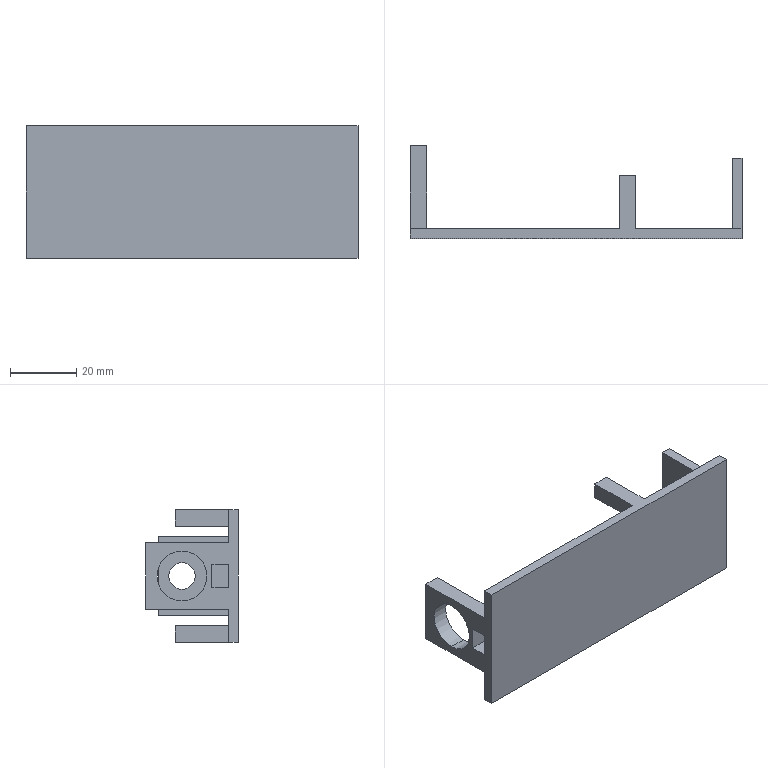Part | SolidWorks | features ICE 5, Extrusion 1 | 1 solid | 29 faces | box 100 x 28 x 40 mm | volume 15612 mm3 | plane 25 | cylinder 4 | commonest cylinder face diameters 8 x2 15 x2
STEP:
#1=CARTESIAN_POINT('',(47.,17.,4.));
#2=VERTEX_POINT('',#1);
#3=CARTESIAN_POINT('',(47.,17.,-4.));
#4=VERTEX_POINT('',#3);
#5=CARTESIAN_POINT('',(47.,17.,0.));
#6=DIRECTION('',(1.,0.,0.));
#7=DIRECTION('',(0.,0.,-1.));
#8=AXIS2_PLACEMENT_3D('',#5,#6,#7);
#9=CIRCLE('',#8,4.);
#10=EDGE_CURVE('',#2,#4,#9,.T.);
#11=ORIENTED_EDGE('',*,*,#10,.F.);
#12=CARTESIAN_POINT('',(50.,17.,4.));
#13=VERTEX_POINT('',#12);
#14=CARTESIAN_POINT('',(47.,17.,4.));
#15=DIRECTION('',(1.,0.,0.));
#16=VECTOR('',#15,1000.);
#17=LINE('',#14,#16);
#18=EDGE_CURVE('',#2,#13,#17,.T.);
#19=ORIENTED_EDGE('',*,*,#18,.T.);
#20=CARTESIAN_POINT('',(50.,17.,-4.));
#21=VERTEX_POINT('',#20);
#22=CARTESIAN_POINT('',(50.,17.,0.));
#23=DIRECTION('',(1.,0.,0.));
#24=DIRECTION('',(0.,0.,-1.));
#25=AXIS2_PLACEMENT_3D('',#22,#23,#24);
#26=CIRCLE('',#25,4.);
#27=EDGE_CURVE('',#13,#21,#26,.T.);
#28=ORIENTED_EDGE('',*,*,#27,.T.);
#29=CARTESIAN_POINT('',(47.,17.,-4.));
#30=DIRECTION('',(1.,0.,0.));
#31=VECTOR('',#30,1000.);
#32=LINE('',#29,#31);
#33=EDGE_CURVE('',#4,#21,#32,.T.);
#34=ORIENTED_EDGE('',*,*,#33,.F.);
#35=EDGE_LOOP('',(#11,#19,#28,#34));
#36=FACE_OUTER_BOUND('',#35,.T.);
#37=CARTESIAN_POINT('',(47.,17.,0.));
#38=DIRECTION('',(1.,0.,0.));
#39=DIRECTION('',(0.,0.,-1.));
#40=AXIS2_PLACEMENT_3D('',#37,#38,#39);
#41=CYLINDRICAL_SURFACE('',#40,4.);
#42=ADVANCED_FACE('',(#36),#41,.F.);
#43=CARTESIAN_POINT('',(-45.,17.,-7.5));
#44=VERTEX_POINT('',#43);
#45=CARTESIAN_POINT('',(-45.,17.,7.5));
#46=VERTEX_POINT('',#45);
#47=CARTESIAN_POINT('',(-45.,17.,0.));
#48=DIRECTION('',(-1.,0.,0.));
#49=DIRECTION('',(0.,0.,1.));
#50=AXIS2_PLACEMENT_3D('',#47,#48,#49);
#51=CIRCLE('',#50,7.5);
#52=EDGE_CURVE('',#44,#46,#51,.T.);
#53=ORIENTED_EDGE('',*,*,#52,.F.);
#54=CARTESIAN_POINT('',(-50.,17.,-7.5));
#55=VERTEX_POINT('',#54);
#56=CARTESIAN_POINT('',(-45.,17.,-7.5));
#57=DIRECTION('',(-1.,0.,0.));
#58=VECTOR('',#57,1000.);
#59=LINE('',#56,#58);
#60=EDGE_CURVE('',#44,#55,#59,.T.);
#61=ORIENTED_EDGE('',*,*,#60,.T.);
#62=CARTESIAN_POINT('',(-50.,17.,7.5));
#63=VERTEX_POINT('',#62);
#64=CARTESIAN_POINT('',(-50.,17.,0.));
#65=DIRECTION('',(-1.,0.,0.));
#66=DIRECTION('',(0.,0.,1.));
#67=AXIS2_PLACEMENT_3D('',#64,#65,#66);
#68=CIRCLE('',#67,7.5);
#69=EDGE_CURVE('',#55,#63,#68,.T.);
#70=ORIENTED_EDGE('',*,*,#69,.T.);
#71=CARTESIAN_POINT('',(-45.,17.,7.5));
#72=DIRECTION('',(-1.,0.,0.));
#73=VECTOR('',#72,1000.);
#74=LINE('',#71,#73);
#75=EDGE_CURVE('',#46,#63,#74,.T.);
#76=ORIENTED_EDGE('',*,*,#75,.F.);
#77=EDGE_LOOP('',(#53,#61,#70,#76));
#78=FACE_OUTER_BOUND('',#77,.T.);
#79=CARTESIAN_POINT('',(-45.,17.,0.));
#80=DIRECTION('',(-1.,0.,0.));
#81=DIRECTION('',(0.,0.,1.));
#82=AXIS2_PLACEMENT_3D('',#79,#80,#81);
#83=CYLINDRICAL_SURFACE('',#82,7.5);
#84=ADVANCED_FACE('',(#78),#83,.F.);
#85=CARTESIAN_POINT('',(50.,3.,20.));
#86=VERTEX_POINT('',#85);
#87=CARTESIAN_POINT('',(50.,3.,12.));
#88=VERTEX_POINT('',#87);
#89=CARTESIAN_POINT('',(50.,3.,20.));
#90=DIRECTION('',(0.,0.,-1.));
#91=VECTOR('',#90,1000.);
#92=LINE('',#89,#91);
#93=EDGE_CURVE('',#86,#88,#92,.T.);
#94=ORIENTED_EDGE('',*,*,#93,.T.);
#95=CARTESIAN_POINT('',(47.,3.,12.));
#96=VERTEX_POINT('',#95);
#97=CARTESIAN_POINT('',(0.,3.,12.));
#98=DIRECTION('',(-1.,0.,0.));
#99=VECTOR('',#98,1000.);
#100=LINE('',#97,#99);
#101=EDGE_CURVE('',#88,#96,#100,.T.);
#102=ORIENTED_EDGE('',*,*,#101,.T.);
#103=CARTESIAN_POINT('',(47.,3.,-12.));
#104=VERTEX_POINT('',#103);
#105=CARTESIAN_POINT('',(47.,3.,0.));
#106=DIRECTION('',(0.,0.,-1.));
#107=VECTOR('',#106,1000.);
#108=LINE('',#105,#107);
#109=EDGE_CURVE('',#96,#104,#108,.T.);
#110=ORIENTED_EDGE('',*,*,#109,.T.);
#111=CARTESIAN_POINT('',(50.,3.,-12.));
#112=VERTEX_POINT('',#111);
#113=CARTESIAN_POINT('',(0.,3.,-12.));
#114=DIRECTION('',(1.,0.,0.));
#115=VECTOR('',#114,1000.);
#116=LINE('',#113,#115);
#117=EDGE_CURVE('',#104,#112,#116,.T.);
#118=ORIENTED_EDGE('',*,*,#117,.T.);
#119=CARTESIAN_POINT('',(50.,3.,-20.));
#120=VERTEX_POINT('',#119);
#121=CARTESIAN_POINT('',(50.,3.,20.));
#122=DIRECTION('',(0.,0.,-1.));
#123=VECTOR('',#122,1000.);
#124=LINE('',#121,#123);
#125=EDGE_CURVE('',#112,#120,#124,.T.);
#126=ORIENTED_EDGE('',*,*,#125,.T.);
#127=CARTESIAN_POINT('',(18.,3.,-20.));
#128=VERTEX_POINT('',#127);
#129=CARTESIAN_POINT('',(-50.,3.,-20.));
#130=DIRECTION('',(-1.,0.,0.));
#131=VECTOR('',#130,1000.);
#132=LINE('',#129,#131);
#133=EDGE_CURVE('',#120,#128,#132,.T.);
#134=ORIENTED_EDGE('',*,*,#133,.T.);
#135=CARTESIAN_POINT('',(18.,3.,-15.));
#136=VERTEX_POINT('',#135);
#137=CARTESIAN_POINT('',(18.,3.,-20.));
#138=DIRECTION('',(0.,0.,-1.));
#139=VECTOR('',#138,1000.);
#140=LINE('',#137,#139);
#141=EDGE_CURVE('',#136,#128,#140,.T.);
#142=ORIENTED_EDGE('',*,*,#141,.F.);
#143=CARTESIAN_POINT('',(13.,3.,-15.));
#144=VERTEX_POINT('',#143);
#145=CARTESIAN_POINT('',(18.,3.,-15.));
#146=DIRECTION('',(-1.,0.,0.));
#147=VECTOR('',#146,1000.);
#148=LINE('',#145,#147);
#149=EDGE_CURVE('',#136,#144,#148,.T.);
#150=ORIENTED_EDGE('',*,*,#149,.T.);
#151=CARTESIAN_POINT('',(13.,3.,-20.));
#152=VERTEX_POINT('',#151);
#153=CARTESIAN_POINT('',(13.,3.,-20.));
#154=DIRECTION('',(0.,0.,-1.));
#155=VECTOR('',#154,1000.);
#156=LINE('',#153,#155);
#157=EDGE_CURVE('',#144,#152,#156,.T.);
#158=ORIENTED_EDGE('',*,*,#157,.T.);
#159=CARTESIAN_POINT('',(-50.,3.,-20.));
#160=VERTEX_POINT('',#159);
#161=CARTESIAN_POINT('',(-50.,3.,-20.));
#162=DIRECTION('',(-1.,0.,0.));
#163=VECTOR('',#162,1000.);
#164=LINE('',#161,#163);
#165=EDGE_CURVE('',#152,#160,#164,.T.);
#166=ORIENTED_EDGE('',*,*,#165,.T.);
#167=CARTESIAN_POINT('',(-50.,3.,-10.));
#168=VERTEX_POINT('',#167);
#169=CARTESIAN_POINT('',(-50.,3.,20.));
#170=DIRECTION('',(0.,0.,1.));
#171=VECTOR('',#170,1000.);
#172=LINE('',#169,#171);
#173=EDGE_CURVE('',#160,#168,#172,.T.);
#174=ORIENTED_EDGE('',*,*,#173,.T.);
#175=CARTESIAN_POINT('',(-45.,3.,-10.));
#176=VERTEX_POINT('',#175);
#177=CARTESIAN_POINT('',(-45.,3.,-10.));
#178=DIRECTION('',(-1.,0.,0.));
#179=VECTOR('',#178,1000.);
#180=LINE('',#177,#179);
#181=EDGE_CURVE('',#176,#168,#180,.T.);
#182=ORIENTED_EDGE('',*,*,#181,.F.);
#183=CARTESIAN_POINT('',(-45.,3.,-3.5));
#184=VERTEX_POINT('',#183);
#185=CARTESIAN_POINT('',(-45.,3.,-10.));
#186=DIRECTION('',(0.,0.,1.));
#187=VECTOR('',#186,1000.);
#188=LINE('',#185,#187);
#189=EDGE_CURVE('',#176,#184,#188,.T.);
#190=ORIENTED_EDGE('',*,*,#189,.T.);
#191=CARTESIAN_POINT('',(-50.,3.,-3.5));
#192=VERTEX_POINT('',#191);
#193=CARTESIAN_POINT('',(-45.,3.,-3.5));
#194=DIRECTION('',(-1.,0.,0.));
#195=VECTOR('',#194,1000.);
#196=LINE('',#193,#195);
#197=EDGE_CURVE('',#184,#192,#196,.T.);
#198=ORIENTED_EDGE('',*,*,#197,.T.);
#199=CARTESIAN_POINT('',(-50.,3.,3.5));
#200=VERTEX_POINT('',#199);
#201=CARTESIAN_POINT('',(-50.,3.,20.));
#202=DIRECTION('',(0.,0.,1.));
#203=VECTOR('',#202,1000.);
#204=LINE('',#201,#203);
#205=EDGE_CURVE('',#192,#200,#204,.T.);
#206=ORIENTED_EDGE('',*,*,#205,.T.);
#207=CARTESIAN_POINT('',(-45.,3.,3.5));
#208=VERTEX_POINT('',#207);
#209=CARTESIAN_POINT('',(-45.,3.,3.5));
#210=DIRECTION('',(-1.,0.,0.));
#211=VECTOR('',#210,1000.);
#212=LINE('',#209,#211);
#213=EDGE_CURVE('',#208,#200,#212,.T.);
#214=ORIENTED_EDGE('',*,*,#213,.F.);
#215=CARTESIAN_POINT('',(-45.,3.,10.));
#216=VERTEX_POINT('',#215);
#217=CARTESIAN_POINT('',(-45.,3.,10.));
#218=DIRECTION('',(0.,0.,1.));
#219=VECTOR('',#218,1000.);
#220=LINE('',#217,#219);
#221=EDGE_CURVE('',#208,#216,#220,.T.);
#222=ORIENTED_EDGE('',*,*,#221,.T.);
#223=CARTESIAN_POINT('',(-50.,3.,10.));
#224=VERTEX_POINT('',#223);
#225=CARTESIAN_POINT('',(-45.,3.,10.));
#226=DIRECTION('',(-1.,0.,0.));
#227=VECTOR('',#226,1000.);
#228=LINE('',#225,#227);
#229=EDGE_CURVE('',#216,#224,#228,.T.);
#230=ORIENTED_EDGE('',*,*,#229,.T.);
#231=CARTESIAN_POINT('',(-50.,3.,20.));
#232=VERTEX_POINT('',#231);
#233=CARTESIAN_POINT('',(-50.,3.,20.));
#234=DIRECTION('',(0.,0.,1.));
#235=VECTOR('',#234,1000.);
#236=LINE('',#233,#235);
#237=EDGE_CURVE('',#224,#232,#236,.T.);
#238=ORIENTED_EDGE('',*,*,#237,.T.);
#239=CARTESIAN_POINT('',(13.,3.,20.));
#240=VERTEX_POINT('',#239);
#241=CARTESIAN_POINT('',(-50.,3.,20.));
#242=DIRECTION('',(1.,0.,0.));
#243=VECTOR('',#242,1000.);
#244=LINE('',#241,#243);
#245=EDGE_CURVE('',#232,#240,#244,.T.);
#246=ORIENTED_EDGE('',*,*,#245,.T.);
#247=CARTESIAN_POINT('',(13.,3.,15.));
#248=VERTEX_POINT('',#247);
#249=CARTESIAN_POINT('',(13.,3.,20.));
#250=DIRECTION('',(0.,0.,-1.));
#251=VECTOR('',#250,1000.);
#252=LINE('',#249,#251);
#253=EDGE_CURVE('',#240,#248,#252,.T.);
#254=ORIENTED_EDGE('',*,*,#253,.T.);
#255=CARTESIAN_POINT('',(18.,3.,15.));
#256=VERTEX_POINT('',#255);
#257=CARTESIAN_POINT('',(18.,3.,15.));
#258=DIRECTION('',(-1.,0.,0.));
#259=VECTOR('',#258,1000.);
#260=LINE('',#257,#259);
#261=EDGE_CURVE('',#256,#248,#260,.T.);
#262=ORIENTED_EDGE('',*,*,#261,.F.);
#263=CARTESIAN_POINT('',(18.,3.,20.));
#264=VERTEX_POINT('',#263);
#265=CARTESIAN_POINT('',(18.,3.,20.));
#266=DIRECTION('',(0.,0.,-1.));
#267=VECTOR('',#266,1000.);
#268=LINE('',#265,#267);
#269=EDGE_CURVE('',#264,#256,#268,.T.);
#270=ORIENTED_EDGE('',*,*,#269,.F.);
#271=CARTESIAN_POINT('',(-50.,3.,20.));
#272=DIRECTION('',(1.,0.,0.));
#273=VECTOR('',#272,1000.);
#274=LINE('',#271,#273);
#275=EDGE_CURVE('',#264,#86,#274,.T.);
#276=ORIENTED_EDGE('',*,*,#275,.T.);
#277=EDGE_LOOP('',(#94,#102,#110,#118,#126,#134,#142,#150,#158,#166,#174,#182,#190,#198,#206,#214,#222,#230,#238,#246,#254,#262,#270,#276));
#278=FACE_OUTER_BOUND('',#277,.T.);
#279=CARTESIAN_POINT('',(0.,3.,0.));
#280=DIRECTION('',(0.,-1.,0.));
#281=DIRECTION('',(0.,0.,-1.));
#282=AXIS2_PLACEMENT_3D('',#279,#280,#281);
#283=PLANE('',#282);
#284=ADVANCED_FACE('',(#278),#283,.F.);
#285=ORIENTED_EDGE('',*,*,#125,.F.);
#286=CARTESIAN_POINT('',(50.,24.132,-12.));
#287=VERTEX_POINT('',#286);
#288=CARTESIAN_POINT('',(50.,24.132,-12.));
#289=DIRECTION('',(0.,1.,0.));
#290=VECTOR('',#289,1000.);
#291=LINE('',#288,#290);
#292=EDGE_CURVE('',#112,#287,#291,.T.);
#293=ORIENTED_EDGE('',*,*,#292,.T.);
#294=CARTESIAN_POINT('',(50.,24.132,12.));
#295=VERTEX_POINT('',#294);
#296=CARTESIAN_POINT('',(50.,24.132,12.));
#297=DIRECTION('',(0.,0.,1.));
#298=VECTOR('',#297,1000.);
#299=LINE('',#296,#298);
#300=EDGE_CURVE('',#287,#295,#299,.T.);
#301=ORIENTED_EDGE('',*,*,#300,.T.);
#302=CARTESIAN_POINT('',(50.,0.,12.));
#303=DIRECTION('',(0.,-1.,0.));
#304=VECTOR('',#303,1000.);
#305=LINE('',#302,#304);
#306=EDGE_CURVE('',#295,#88,#305,.T.);
#307=ORIENTED_EDGE('',*,*,#306,.T.);
#308=ORIENTED_EDGE('',*,*,#93,.F.);
#309=CARTESIAN_POINT('',(50.,0.,20.));
#310=VERTEX_POINT('',#309);
#311=CARTESIAN_POINT('',(50.,3.,20.));
#312=DIRECTION('',(0.,-1.,0.));
#313=VECTOR('',#312,1000.);
#314=LINE('',#311,#313);
#315=EDGE_CURVE('',#86,#310,#314,.T.);
#316=ORIENTED_EDGE('',*,*,#315,.T.);
#317=CARTESIAN_POINT('',(50.,0.,-20.));
#318=VERTEX_POINT('',#317);
#319=CARTESIAN_POINT('',(50.,0.,20.));
#320=DIRECTION('',(0.,0.,-1.));
#321=VECTOR('',#320,1000.);
#322=LINE('',#319,#321);
#323=EDGE_CURVE('',#310,#318,#322,.T.);
#324=ORIENTED_EDGE('',*,*,#323,.T.);
#325=CARTESIAN_POINT('',(50.,3.,-20.));
#326=DIRECTION('',(0.,-1.,0.));
#327=VECTOR('',#326,1000.);
#328=LINE('',#325,#327);
#329=EDGE_CURVE('',#120,#318,#328,.T.);
#330=ORIENTED_EDGE('',*,*,#329,.F.);
#331=EDGE_LOOP('',(#285,#293,#301,#307,#308,#316,#324,#330));
#332=FACE_OUTER_BOUND('',#331,.T.);
#333=CARTESIAN_POINT('',(50.,17.,0.));
#334=DIRECTION('',(1.,0.,0.));
#335=DIRECTION('',(0.,0.,-1.));
#336=AXIS2_PLACEMENT_3D('',#333,#334,#335);
#337=CIRCLE('',#336,4.);
#338=EDGE_CURVE('',#21,#13,#337,.T.);
#339=ORIENTED_EDGE('',*,*,#338,.F.);
#340=ORIENTED_EDGE('',*,*,#27,.F.);
#341=EDGE_LOOP('',(#339,#340));
#342=FACE_BOUND('',#341,.T.);
#343=CARTESIAN_POINT('',(50.,3.,20.));
#344=DIRECTION('',(-1.,0.,0.));
#345=DIRECTION('',(0.,0.,1.));
#346=AXIS2_PLACEMENT_3D('',#343,#344,#345);
#347=PLANE('',#346);
#348=ADVANCED_FACE('',(#332,#342),#347,.F.);
#349=CARTESIAN_POINT('',(-50.,0.,-20.));
#350=VERTEX_POINT('',#349);
#351=CARTESIAN_POINT('',(-50.,0.,-20.));
#352=DIRECTION('',(-1.,0.,0.));
#353=VECTOR('',#352,1000.);
#354=LINE('',#351,#353);
#355=EDGE_CURVE('',#318,#350,#354,.T.);
#356=ORIENTED_EDGE('',*,*,#355,.T.);
#357=CARTESIAN_POINT('',(-50.,3.,-20.));
#358=DIRECTION('',(0.,-1.,0.));
#359=VECTOR('',#358,1000.);
#360=LINE('',#357,#359);
#361=EDGE_CURVE('',#160,#350,#360,.T.);
#362=ORIENTED_EDGE('',*,*,#361,.F.);
#363=ORIENTED_EDGE('',*,*,#165,.F.);
#364=CARTESIAN_POINT('',(13.,19.,-20.));
#365=VERTEX_POINT('',#364);
#366=CARTESIAN_POINT('',(13.,3.,-20.));
#367=DIRECTION('',(0.,1.,0.));
#368=VECTOR('',#367,1000.);
#369=LINE('',#366,#368);
#370=EDGE_CURVE('',#152,#365,#369,.T.);
#371=ORIENTED_EDGE('',*,*,#370,.T.);
#372=CARTESIAN_POINT('',(18.,19.,-20.));
#373=VERTEX_POINT('',#372);
#374=CARTESIAN_POINT('',(18.,19.,-20.));
#375=DIRECTION('',(-1.,0.,0.));
#376=VECTOR('',#375,1000.);
#377=LINE('',#374,#376);
#378=EDGE_CURVE('',#373,#365,#377,.T.);
#379=ORIENTED_EDGE('',*,*,#378,.F.);
#380=CARTESIAN_POINT('',(18.,3.,-20.));
#381=DIRECTION('',(0.,1.,0.));
#382=VECTOR('',#381,1000.);
#383=LINE('',#380,#382);
#384=EDGE_CURVE('',#128,#373,#383,.T.);
#385=ORIENTED_EDGE('',*,*,#384,.F.);
#386=ORIENTED_EDGE('',*,*,#133,.F.);
#387=ORIENTED_EDGE('',*,*,#329,.T.);
#388=EDGE_LOOP('',(#356,#362,#363,#371,#379,#385,#386,#387));
#389=FACE_OUTER_BOUND('',#388,.T.);
#390=CARTESIAN_POINT('',(-50.,3.,-20.));
#391=DIRECTION('',(0.,0.,1.));
#392=DIRECTION('',(1.,0.,0.));
#393=AXIS2_PLACEMENT_3D('',#390,#391,#392);
#394=PLANE('',#393);
#395=ADVANCED_FACE('',(#389),#394,.F.);
#396=ORIENTED_EDGE('',*,*,#237,.F.);
#397=CARTESIAN_POINT('',(-50.,28.,10.));
#398=VERTEX_POINT('',#397);
#399=CARTESIAN_POINT('',(-50.,3.,10.));
#400=DIRECTION('',(0.,1.,0.));
#401=VECTOR('',#400,1000.);
#402=LINE('',#399,#401);
#403=EDGE_CURVE('',#224,#398,#402,.T.);
#404=ORIENTED_EDGE('',*,*,#403,.T.);
#405=CARTESIAN_POINT('',(-50.,28.,-10.));
#406=VERTEX_POINT('',#405);
#407=CARTESIAN_POINT('',(-50.,28.,10.));
#408=DIRECTION('',(0.,0.,-1.));
#409=VECTOR('',#408,1000.);
#410=LINE('',#407,#409);
#411=EDGE_CURVE('',#398,#406,#410,.T.);
#412=ORIENTED_EDGE('',*,*,#411,.T.);
#413=CARTESIAN_POINT('',(-50.,28.,-10.));
#414=DIRECTION('',(0.,-1.,0.));
#415=VECTOR('',#414,1000.);
#416=LINE('',#413,#415);
#417=EDGE_CURVE('',#406,#168,#416,.T.);
#418=ORIENTED_EDGE('',*,*,#417,.T.);
#419=ORIENTED_EDGE('',*,*,#173,.F.);
#420=ORIENTED_EDGE('',*,*,#361,.T.);
#421=CARTESIAN_POINT('',(-50.,0.,20.));
#422=VERTEX_POINT('',#421);
#423=CARTESIAN_POINT('',(-50.,0.,20.));
#424=DIRECTION('',(0.,0.,1.));
#425=VECTOR('',#424,1000.);
#426=LINE('',#423,#425);
#427=EDGE_CURVE('',#350,#422,#426,.T.);
#428=ORIENTED_EDGE('',*,*,#427,.T.);
#429=CARTESIAN_POINT('',(-50.,3.,20.));
#430=DIRECTION('',(0.,-1.,0.));
#431=VECTOR('',#430,1000.);
#432=LINE('',#429,#431);
#433=EDGE_CURVE('',#232,#422,#432,.T.);
#434=ORIENTED_EDGE('',*,*,#433,.F.);
#435=EDGE_LOOP('',(#396,#404,#412,#418,#419,#420,#428,#434));
#436=FACE_OUTER_BOUND('',#435,.T.);
#437=CARTESIAN_POINT('',(-50.,8.,3.5));
#438=VERTEX_POINT('',#437);
#439=CARTESIAN_POINT('',(-50.,8.,3.5));
#440=DIRECTION('',(0.,-1.,0.));
#441=VECTOR('',#440,1000.);
#442=LINE('',#439,#441);
#443=EDGE_CURVE('',#438,#200,#442,.T.);
#444=ORIENTED_EDGE('',*,*,#443,.T.);
#445=ORIENTED_EDGE('',*,*,#205,.F.);
#446=CARTESIAN_POINT('',(-50.,8.,-3.5));
#447=VERTEX_POINT('',#446);
#448=CARTESIAN_POINT('',(-50.,3.,-3.5));
#449=DIRECTION('',(0.,1.,0.));
#450=VECTOR('',#449,1000.);
#451=LINE('',#448,#450);
#452=EDGE_CURVE('',#192,#447,#451,.T.);
#453=ORIENTED_EDGE('',*,*,#452,.T.);
#454=CARTESIAN_POINT('',(-50.,8.,-3.5));
#455=DIRECTION('',(0.,0.,1.));
#456=VECTOR('',#455,1000.);
#457=LINE('',#454,#456);
#458=EDGE_CURVE('',#447,#438,#457,.T.);
#459=ORIENTED_EDGE('',*,*,#458,.T.);
#460=EDGE_LOOP('',(#444,#445,#453,#459));
#461=FACE_BOUND('',#460,.T.);
#462=CARTESIAN_POINT('',(-50.,17.,0.));
#463=DIRECTION('',(-1.,0.,0.));
#464=DIRECTION('',(0.,0.,1.));
#465=AXIS2_PLACEMENT_3D('',#462,#463,#464);
#466=CIRCLE('',#465,7.5);
#467=EDGE_CURVE('',#63,#55,#466,.T.);
#468=ORIENTED_EDGE('',*,*,#467,.F.);
#469=ORIENTED_EDGE('',*,*,#69,.F.);
#470=EDGE_LOOP('',(#468,#469));
#471=FACE_BOUND('',#470,.T.);
#472=CARTESIAN_POINT('',(-50.,3.,20.));
#473=DIRECTION('',(1.,0.,0.));
#474=DIRECTION('',(0.,0.,-1.));
#475=AXIS2_PLACEMENT_3D('',#472,#473,#474);
#476=PLANE('',#475);
#477=ADVANCED_FACE('',(#436,#461,#471),#476,.F.);
#478=CARTESIAN_POINT('',(-50.,0.,20.));
#479=DIRECTION('',(1.,0.,0.));
#480=VECTOR('',#479,1000.);
#481=LINE('',#478,#480);
#482=EDGE_CURVE('',#422,#310,#481,.T.);
#483=ORIENTED_EDGE('',*,*,#482,.T.);
#484=ORIENTED_EDGE('',*,*,#315,.F.);
#485=ORIENTED_EDGE('',*,*,#275,.F.);
#486=CARTESIAN_POINT('',(18.,19.,20.));
#487=VERTEX_POINT('',#486);
#488=CARTESIAN_POINT('',(18.,3.,20.));
#489=DIRECTION('',(0.,-1.,0.));
#490=VECTOR('',#489,1000.);
#491=LINE('',#488,#490);
#492=EDGE_CURVE('',#487,#264,#491,.T.);
#493=ORIENTED_EDGE('',*,*,#492,.F.);
#494=CARTESIAN_POINT('',(13.,19.,20.));
#495=VERTEX_POINT('',#494);
#496=CARTESIAN_POINT('',(18.,19.,20.));
#497=DIRECTION('',(-1.,0.,0.));
#498=VECTOR('',#497,1000.);
#499=LINE('',#496,#498);
#500=EDGE_CURVE('',#487,#495,#499,.T.);
#501=ORIENTED_EDGE('',*,*,#500,.T.);
#502=CARTESIAN_POINT('',(13.,3.,20.));
#503=DIRECTION('',(0.,-1.,0.));
#504=VECTOR('',#503,1000.);
#505=LINE('',#502,#504);
#506=EDGE_CURVE('',#495,#240,#505,.T.);
#507=ORIENTED_EDGE('',*,*,#506,.T.);
#508=ORIENTED_EDGE('',*,*,#245,.F.);
#509=ORIENTED_EDGE('',*,*,#433,.T.);
#510=EDGE_LOOP('',(#483,#484,#485,#493,#501,#507,#508,#509));
#511=FACE_OUTER_BOUND('',#510,.T.);
#512=CARTESIAN_POINT('',(-50.,3.,20.));
#513=DIRECTION('',(0.,0.,-1.));
#514=DIRECTION('',(-1.,0.,0.));
#515=AXIS2_PLACEMENT_3D('',#512,#513,#514);
#516=PLANE('',#515);
#517=ADVANCED_FACE('',(#511),#516,.F.);
#518=ORIENTED_EDGE('',*,*,#355,.F.);
#519=ORIENTED_EDGE('',*,*,#323,.F.);
#520=ORIENTED_EDGE('',*,*,#482,.F.);
#521=ORIENTED_EDGE('',*,*,#427,.F.);
#522=EDGE_LOOP('',(#518,#519,#520,#521));
#523=FACE_OUTER_BOUND('',#522,.T.);
#524=CARTESIAN_POINT('',(0.,0.,0.));
#525=DIRECTION('',(0.,-1.,0.));
#526=DIRECTION('',(0.,0.,-1.));
#527=AXIS2_PLACEMENT_3D('',#524,#525,#526);
#528=PLANE('',#527);
#529=ADVANCED_FACE('',(#523),#528,.T.);
#530=ORIENTED_EDGE('',*,*,#417,.F.);
#531=CARTESIAN_POINT('',(-45.,28.,-10.));
#532=VERTEX_POINT('',#531);
#533=CARTESIAN_POINT('',(-45.,28.,-10.));
#534=DIRECTION('',(-1.,0.,0.));
#535=VECTOR('',#534,1000.);
#536=LINE('',#533,#535);
#537=EDGE_CURVE('',#532,#406,#536,.T.);
#538=ORIENTED_EDGE('',*,*,#537,.F.);
#539=CARTESIAN_POINT('',(-45.,28.,-10.));
#540=DIRECTION('',(0.,-1.,0.));
#541=VECTOR('',#540,1000.);
#542=LINE('',#539,#541);
#543=EDGE_CURVE('',#532,#176,#542,.T.);
#544=ORIENTED_EDGE('',*,*,#543,.T.);
#545=ORIENTED_EDGE('',*,*,#181,.T.);
#546=EDGE_LOOP('',(#530,#538,#544,#545));
#547=FACE_OUTER_BOUND('',#546,.T.);
#548=CARTESIAN_POINT('',(-45.,28.,-10.));
#549=DIRECTION('',(0.,0.,-1.));
#550=DIRECTION('',(0.,1.,0.));
#551=AXIS2_PLACEMENT_3D('',#548,#549,#550);
#552=PLANE('',#551);
#553=ADVANCED_FACE('',(#547),#552,.T.);
#554=ORIENTED_EDGE('',*,*,#411,.F.);
#555=CARTESIAN_POINT('',(-45.,28.,10.));
#556=VERTEX_POINT('',#555);
#557=CARTESIAN_POINT('',(-45.,28.,10.));
#558=DIRECTION('',(-1.,0.,0.));
#559=VECTOR('',#558,1000.);
#560=LINE('',#557,#559);
#561=EDGE_CURVE('',#556,#398,#560,.T.);
#562=ORIENTED_EDGE('',*,*,#561,.F.);
#563=CARTESIAN_POINT('',(-45.,28.,10.));
#564=DIRECTION('',(0.,0.,-1.));
#565=VECTOR('',#564,1000.);
#566=LINE('',#563,#565);
#567=EDGE_CURVE('',#556,#532,#566,.T.);
#568=ORIENTED_EDGE('',*,*,#567,.T.);
#569=ORIENTED_EDGE('',*,*,#537,.T.);
#570=EDGE_LOOP('',(#554,#562,#568,#569));
#571=FACE_OUTER_BOUND('',#570,.T.);
#572=CARTESIAN_POINT('',(-45.,28.,10.));
#573=DIRECTION('',(0.,1.,0.));
#574=DIRECTION('',(0.,0.,1.));
#575=AXIS2_PLACEMENT_3D('',#572,#573,#574);
#576=PLANE('',#575);
#577=ADVANCED_FACE('',(#571),#576,.T.);
#578=ORIENTED_EDGE('',*,*,#403,.F.);
#579=ORIENTED_EDGE('',*,*,#229,.F.);
#580=CARTESIAN_POINT('',(-45.,3.,10.));
#581=DIRECTION('',(0.,1.,0.));
#582=VECTOR('',#581,1000.);
#583=LINE('',#580,#582);
#584=EDGE_CURVE('',#216,#556,#583,.T.);
#585=ORIENTED_EDGE('',*,*,#584,.T.);
#586=ORIENTED_EDGE('',*,*,#561,.T.);
#587=EDGE_LOOP('',(#578,#579,#585,#586));
#588=FACE_OUTER_BOUND('',#587,.T.);
#589=CARTESIAN_POINT('',(-45.,3.,10.));
#590=DIRECTION('',(0.,0.,1.));
#591=DIRECTION('',(0.,-1.,0.));
#592=AXIS2_PLACEMENT_3D('',#589,#590,#591);
#593=PLANE('',#592);
#594=ADVANCED_FACE('',(#588),#593,.T.);
#595=ORIENTED_EDGE('',*,*,#443,.F.);
#596=CARTESIAN_POINT('',(-45.,8.,3.5));
#597=VERTEX_POINT('',#596);
#598=CARTESIAN_POINT('',(-45.,8.,3.5));
#599=DIRECTION('',(-1.,0.,0.));
#600=VECTOR('',#599,1000.);
#601=LINE('',#598,#600);
#602=EDGE_CURVE('',#597,#438,#601,.T.);
#603=ORIENTED_EDGE('',*,*,#602,.F.);
#604=CARTESIAN_POINT('',(-45.,8.,3.5));
#605=DIRECTION('',(0.,-1.,0.));
#606=VECTOR('',#605,1000.);
#607=LINE('',#604,#606);
#608=EDGE_CURVE('',#597,#208,#607,.T.);
#609=ORIENTED_EDGE('',*,*,#608,.T.);
#610=ORIENTED_EDGE('',*,*,#213,.T.);
#611=EDGE_LOOP('',(#595,#603,#609,#610));
#612=FACE_OUTER_BOUND('',#611,.T.);
#613=CARTESIAN_POINT('',(-45.,8.,3.5));
#614=DIRECTION('',(0.,0.,-1.));
#615=DIRECTION('',(0.,1.,0.));
#616=AXIS2_PLACEMENT_3D('',#613,#614,#615);
#617=PLANE('',#616);
#618=ADVANCED_FACE('',(#612),#617,.T.);
#619=ORIENTED_EDGE('',*,*,#458,.F.);
#620=CARTESIAN_POINT('',(-45.,8.,-3.5));
#621=VERTEX_POINT('',#620);
#622=CARTESIAN_POINT('',(-45.,8.,-3.5));
#623=DIRECTION('',(-1.,0.,0.));
#624=VECTOR('',#623,1000.);
#625=LINE('',#622,#624);
#626=EDGE_CURVE('',#621,#447,#625,.T.);
#627=ORIENTED_EDGE('',*,*,#626,.F.);
#628=CARTESIAN_POINT('',(-45.,8.,-3.5));
#629=DIRECTION('',(0.,0.,1.));
#630=VECTOR('',#629,1000.);
#631=LINE('',#628,#630);
#632=EDGE_CURVE('',#621,#597,#631,.T.);
#633=ORIENTED_EDGE('',*,*,#632,.T.);
#634=ORIENTED_EDGE('',*,*,#602,.T.);
#635=EDGE_LOOP('',(#619,#627,#633,#634));
#636=FACE_OUTER_BOUND('',#635,.T.);
#637=CARTESIAN_POINT('',(-45.,8.,-3.5));
#638=DIRECTION('',(0.,-1.,0.));
#639=DIRECTION('',(0.,0.,-1.));
#640=AXIS2_PLACEMENT_3D('',#637,#638,#639);
#641=PLANE('',#640);
#642=ADVANCED_FACE('',(#636),#641,.T.);
#643=ORIENTED_EDGE('',*,*,#452,.F.);
#644=ORIENTED_EDGE('',*,*,#197,.F.);
#645=CARTESIAN_POINT('',(-45.,3.,-3.5));
#646=DIRECTION('',(0.,1.,0.));
#647=VECTOR('',#646,1000.);
#648=LINE('',#645,#647);
#649=EDGE_CURVE('',#184,#621,#648,.T.);
#650=ORIENTED_EDGE('',*,*,#649,.T.);
#651=ORIENTED_EDGE('',*,*,#626,.T.);
#652=EDGE_LOOP('',(#643,#644,#650,#651));
#653=FACE_OUTER_BOUND('',#652,.T.);
#654=CARTESIAN_POINT('',(-45.,3.,-3.5));
#655=DIRECTION('',(0.,0.,1.));
#656=DIRECTION('',(0.,-1.,0.));
#657=AXIS2_PLACEMENT_3D('',#654,#655,#656);
#658=PLANE('',#657);
#659=ADVANCED_FACE('',(#653),#658,.T.);
#660=CARTESIAN_POINT('',(-45.,17.,0.));
#661=DIRECTION('',(-1.,0.,0.));
#662=DIRECTION('',(0.,0.,1.));
#663=AXIS2_PLACEMENT_3D('',#660,#661,#662);
#664=CIRCLE('',#663,7.5);
#665=EDGE_CURVE('',#46,#44,#664,.T.);
#666=ORIENTED_EDGE('',*,*,#665,.T.);
#667=ORIENTED_EDGE('',*,*,#52,.T.);
#668=EDGE_LOOP('',(#666,#667));
#669=FACE_BOUND('',#668,.T.);
#670=ORIENTED_EDGE('',*,*,#543,.F.);
#671=ORIENTED_EDGE('',*,*,#567,.F.);
#672=ORIENTED_EDGE('',*,*,#584,.F.);
#673=ORIENTED_EDGE('',*,*,#221,.F.);
#674=ORIENTED_EDGE('',*,*,#608,.F.);
#675=ORIENTED_EDGE('',*,*,#632,.F.);
#676=ORIENTED_EDGE('',*,*,#649,.F.);
#677=ORIENTED_EDGE('',*,*,#189,.F.);
#678=EDGE_LOOP('',(#670,#671,#672,#673,#674,#675,#676,#677));
#679=FACE_OUTER_BOUND('',#678,.T.);
#680=CARTESIAN_POINT('',(-45.,0.,0.));
#681=DIRECTION('',(-1.,0.,0.));
#682=DIRECTION('',(0.,0.,1.));
#683=AXIS2_PLACEMENT_3D('',#680,#681,#682);
#684=PLANE('',#683);
#685=ADVANCED_FACE('',(#669,#679),#684,.F.);
#686=ORIENTED_EDGE('',*,*,#60,.F.);
#687=ORIENTED_EDGE('',*,*,#665,.F.);
#688=ORIENTED_EDGE('',*,*,#75,.T.);
#689=ORIENTED_EDGE('',*,*,#467,.T.);
#690=EDGE_LOOP('',(#686,#687,#688,#689));
#691=FACE_OUTER_BOUND('',#690,.T.);
#692=CARTESIAN_POINT('',(-45.,17.,0.));
#693=DIRECTION('',(-1.,0.,0.));
#694=DIRECTION('',(0.,0.,1.));
#695=AXIS2_PLACEMENT_3D('',#692,#693,#694);
#696=CYLINDRICAL_SURFACE('',#695,7.5);
#697=ADVANCED_FACE('',(#691),#696,.F.);
#698=CARTESIAN_POINT('',(13.,19.,-15.));
#699=VERTEX_POINT('',#698);
#700=CARTESIAN_POINT('',(13.,19.,-20.));
#701=DIRECTION('',(0.,0.,1.));
#702=VECTOR('',#701,1000.);
#703=LINE('',#700,#702);
#704=EDGE_CURVE('',#365,#699,#703,.T.);
#705=ORIENTED_EDGE('',*,*,#704,.T.);
#706=CARTESIAN_POINT('',(18.,19.,-15.));
#707=VERTEX_POINT('',#706);
#708=CARTESIAN_POINT('',(18.,19.,-15.));
#709=DIRECTION('',(-1.,0.,0.));
#710=VECTOR('',#709,1000.);
#711=LINE('',#708,#710);
#712=EDGE_CURVE('',#707,#699,#711,.T.);
#713=ORIENTED_EDGE('',*,*,#712,.F.);
#714=CARTESIAN_POINT('',(18.,19.,-20.));
#715=DIRECTION('',(0.,0.,1.));
#716=VECTOR('',#715,1000.);
#717=LINE('',#714,#716);
#718=EDGE_CURVE('',#373,#707,#717,.T.);
#719=ORIENTED_EDGE('',*,*,#718,.F.);
#720=ORIENTED_EDGE('',*,*,#378,.T.);
#721=EDGE_LOOP('',(#705,#713,#719,#720));
#722=FACE_OUTER_BOUND('',#721,.T.);
#723=CARTESIAN_POINT('',(18.,19.,-20.));
#724=DIRECTION('',(0.,-1.,0.));
#725=DIRECTION('',(0.,0.,-1.));
#726=AXIS2_PLACEMENT_3D('',#723,#724,#725);
#727=PLANE('',#726);
#728=ADVANCED_FACE('',(#722),#727,.F.);
#729=CARTESIAN_POINT('',(13.,3.,-15.));
#730=DIRECTION('',(0.,-1.,0.));
#731=VECTOR('',#730,1000.);
#732=LINE('',#729,#731);
#733=EDGE_CURVE('',#699,#144,#732,.T.);
#734=ORIENTED_EDGE('',*,*,#733,.T.);
#735=ORIENTED_EDGE('',*,*,#149,.F.);
#736=CARTESIAN_POINT('',(18.,3.,-15.));
#737=DIRECTION('',(0.,-1.,0.));
#738=VECTOR('',#737,1000.);
#739=LINE('',#736,#738);
#740=EDGE_CURVE('',#707,#136,#739,.T.);
#741=ORIENTED_EDGE('',*,*,#740,.F.);
#742=ORIENTED_EDGE('',*,*,#712,.T.);
#743=EDGE_LOOP('',(#734,#735,#741,#742));
#744=FACE_OUTER_BOUND('',#743,.T.);
#745=CARTESIAN_POINT('',(18.,3.,-15.));
#746=DIRECTION('',(0.,0.,-1.));
#747=DIRECTION('',(-1.,0.,0.));
#748=AXIS2_PLACEMENT_3D('',#745,#746,#747);
#749=PLANE('',#748);
#750=ADVANCED_FACE('',(#744),#749,.F.);
#751=ORIENTED_EDGE('',*,*,#384,.T.);
#752=ORIENTED_EDGE('',*,*,#718,.T.);
#753=ORIENTED_EDGE('',*,*,#740,.T.);
#754=ORIENTED_EDGE('',*,*,#141,.T.);
#755=EDGE_LOOP('',(#751,#752,#753,#754));
#756=FACE_OUTER_BOUND('',#755,.T.);
#757=CARTESIAN_POINT('',(18.,0.,0.));
#758=DIRECTION('',(1.,0.,0.));
#759=DIRECTION('',(0.,0.,-1.));
#760=AXIS2_PLACEMENT_3D('',#757,#758,#759);
#761=PLANE('',#760);
#762=ADVANCED_FACE('',(#756),#761,.T.);
#763=ORIENTED_EDGE('',*,*,#370,.F.);
#764=ORIENTED_EDGE('',*,*,#157,.F.);
#765=ORIENTED_EDGE('',*,*,#733,.F.);
#766=ORIENTED_EDGE('',*,*,#704,.F.);
#767=EDGE_LOOP('',(#763,#764,#765,#766));
#768=FACE_OUTER_BOUND('',#767,.T.);
#769=CARTESIAN_POINT('',(13.,0.,0.));
#770=DIRECTION('',(1.,0.,0.));
#771=DIRECTION('',(0.,0.,-1.));
#772=AXIS2_PLACEMENT_3D('',#769,#770,#771);
#773=PLANE('',#772);
#774=ADVANCED_FACE('',(#768),#773,.F.);
#775=CARTESIAN_POINT('',(13.,19.,15.));
#776=VERTEX_POINT('',#775);
#777=CARTESIAN_POINT('',(13.,3.,15.));
#778=DIRECTION('',(0.,1.,0.));
#779=VECTOR('',#778,1000.);
#780=LINE('',#777,#779);
#781=EDGE_CURVE('',#248,#776,#780,.T.);
#782=ORIENTED_EDGE('',*,*,#781,.T.);
#783=CARTESIAN_POINT('',(18.,19.,15.));
#784=VERTEX_POINT('',#783);
#785=CARTESIAN_POINT('',(18.,19.,15.));
#786=DIRECTION('',(-1.,0.,0.));
#787=VECTOR('',#786,1000.);
#788=LINE('',#785,#787);
#789=EDGE_CURVE('',#784,#776,#788,.T.);
#790=ORIENTED_EDGE('',*,*,#789,.F.);
#791=CARTESIAN_POINT('',(18.,3.,15.));
#792=DIRECTION('',(0.,1.,0.));
#793=VECTOR('',#792,1000.);
#794=LINE('',#791,#793);
#795=EDGE_CURVE('',#256,#784,#794,.T.);
#796=ORIENTED_EDGE('',*,*,#795,.F.);
#797=ORIENTED_EDGE('',*,*,#261,.T.);
#798=EDGE_LOOP('',(#782,#790,#796,#797));
#799=FACE_OUTER_BOUND('',#798,.T.);
#800=CARTESIAN_POINT('',(18.,3.,15.));
#801=DIRECTION('',(0.,0.,1.));
#802=DIRECTION('',(0.,-1.,0.));
#803=AXIS2_PLACEMENT_3D('',#800,#801,#802);
#804=PLANE('',#803);
#805=ADVANCED_FACE('',(#799),#804,.F.);
#806=CARTESIAN_POINT('',(13.,19.,20.));
#807=DIRECTION('',(0.,0.,1.));
#808=VECTOR('',#807,1000.);
#809=LINE('',#806,#808);
#810=EDGE_CURVE('',#776,#495,#809,.T.);
#811=ORIENTED_EDGE('',*,*,#810,.T.);
#812=ORIENTED_EDGE('',*,*,#500,.F.);
#813=CARTESIAN_POINT('',(18.,19.,20.));
#814=DIRECTION('',(0.,0.,1.));
#815=VECTOR('',#814,1000.);
#816=LINE('',#813,#815);
#817=EDGE_CURVE('',#784,#487,#816,.T.);
#818=ORIENTED_EDGE('',*,*,#817,.F.);
#819=ORIENTED_EDGE('',*,*,#789,.T.);
#820=EDGE_LOOP('',(#811,#812,#818,#819));
#821=FACE_OUTER_BOUND('',#820,.T.);
#822=CARTESIAN_POINT('',(18.,19.,20.));
#823=DIRECTION('',(0.,-1.,0.));
#824=DIRECTION('',(0.,0.,-1.));
#825=AXIS2_PLACEMENT_3D('',#822,#823,#824);
#826=PLANE('',#825);
#827=ADVANCED_FACE('',(#821),#826,.F.);
#828=ORIENTED_EDGE('',*,*,#492,.T.);
#829=ORIENTED_EDGE('',*,*,#269,.T.);
#830=ORIENTED_EDGE('',*,*,#795,.T.);
#831=ORIENTED_EDGE('',*,*,#817,.T.);
#832=EDGE_LOOP('',(#828,#829,#830,#831));
#833=FACE_OUTER_BOUND('',#832,.T.);
#834=CARTESIAN_POINT('',(18.,0.,0.));
#835=DIRECTION('',(-1.,0.,0.));
#836=DIRECTION('',(0.,0.,1.));
#837=AXIS2_PLACEMENT_3D('',#834,#835,#836);
#838=PLANE('',#837);
#839=ADVANCED_FACE('',(#833),#838,.F.);
#840=ORIENTED_EDGE('',*,*,#506,.F.);
#841=ORIENTED_EDGE('',*,*,#810,.F.);
#842=ORIENTED_EDGE('',*,*,#781,.F.);
#843=ORIENTED_EDGE('',*,*,#253,.F.);
#844=EDGE_LOOP('',(#840,#841,#842,#843));
#845=FACE_OUTER_BOUND('',#844,.T.);
#846=CARTESIAN_POINT('',(13.,0.,0.));
#847=DIRECTION('',(-1.,0.,0.));
#848=DIRECTION('',(0.,0.,1.));
#849=AXIS2_PLACEMENT_3D('',#846,#847,#848);
#850=PLANE('',#849);
#851=ADVANCED_FACE('',(#845),#850,.T.);
#852=ORIENTED_EDGE('',*,*,#101,.F.);
#853=ORIENTED_EDGE('',*,*,#306,.F.);
#854=CARTESIAN_POINT('',(47.,24.132,12.));
#855=VERTEX_POINT('',#854);
#856=CARTESIAN_POINT('',(47.,24.132,12.));
#857=DIRECTION('',(1.,0.,0.));
#858=VECTOR('',#857,1000.);
#859=LINE('',#856,#858);
#860=EDGE_CURVE('',#855,#295,#859,.T.);
#861=ORIENTED_EDGE('',*,*,#860,.F.);
#862=CARTESIAN_POINT('',(47.,0.,12.));
#863=DIRECTION('',(0.,-1.,0.));
#864=VECTOR('',#863,1000.);
#865=LINE('',#862,#864);
#866=EDGE_CURVE('',#855,#96,#865,.T.);
#867=ORIENTED_EDGE('',*,*,#866,.T.);
#868=EDGE_LOOP('',(#852,#853,#861,#867));
#869=FACE_OUTER_BOUND('',#868,.T.);
#870=CARTESIAN_POINT('',(47.,0.,12.));
#871=DIRECTION('',(0.,0.,1.));
#872=DIRECTION('',(1.,0.,0.));
#873=AXIS2_PLACEMENT_3D('',#870,#871,#872);
#874=PLANE('',#873);
#875=ADVANCED_FACE('',(#869),#874,.T.);
#876=ORIENTED_EDGE('',*,*,#117,.F.);
#877=CARTESIAN_POINT('',(47.,24.132,-12.));
#878=VERTEX_POINT('',#877);
#879=CARTESIAN_POINT('',(47.,24.132,-12.));
#880=DIRECTION('',(0.,1.,0.));
#881=VECTOR('',#880,1000.);
#882=LINE('',#879,#881);
#883=EDGE_CURVE('',#104,#878,#882,.T.);
#884=ORIENTED_EDGE('',*,*,#883,.T.);
#885=CARTESIAN_POINT('',(47.,24.132,-12.));
#886=DIRECTION('',(1.,0.,0.));
#887=VECTOR('',#886,1000.);
#888=LINE('',#885,#887);
#889=EDGE_CURVE('',#878,#287,#888,.T.);
#890=ORIENTED_EDGE('',*,*,#889,.T.);
#891=ORIENTED_EDGE('',*,*,#292,.F.);
#892=EDGE_LOOP('',(#876,#884,#890,#891));
#893=FACE_OUTER_BOUND('',#892,.T.);
#894=CARTESIAN_POINT('',(47.,24.132,-12.));
#895=DIRECTION('',(0.,0.,-1.));
#896=DIRECTION('',(-1.,0.,0.));
#897=AXIS2_PLACEMENT_3D('',#894,#895,#896);
#898=PLANE('',#897);
#899=ADVANCED_FACE('',(#893),#898,.T.);
#900=CARTESIAN_POINT('',(47.,17.,0.));
#901=DIRECTION('',(1.,0.,0.));
#902=DIRECTION('',(0.,0.,-1.));
#903=AXIS2_PLACEMENT_3D('',#900,#901,#902);
#904=CIRCLE('',#903,4.);
#905=EDGE_CURVE('',#4,#2,#904,.T.);
#906=ORIENTED_EDGE('',*,*,#905,.T.);
#907=ORIENTED_EDGE('',*,*,#10,.T.);
#908=EDGE_LOOP('',(#906,#907));
#909=FACE_BOUND('',#908,.T.);
#910=ORIENTED_EDGE('',*,*,#109,.F.);
#911=ORIENTED_EDGE('',*,*,#866,.F.);
#912=CARTESIAN_POINT('',(47.,24.132,12.));
#913=DIRECTION('',(0.,0.,1.));
#914=VECTOR('',#913,1000.);
#915=LINE('',#912,#914);
#916=EDGE_CURVE('',#878,#855,#915,.T.);
#917=ORIENTED_EDGE('',*,*,#916,.F.);
#918=ORIENTED_EDGE('',*,*,#883,.F.);
#919=EDGE_LOOP('',(#910,#911,#917,#918));
#920=FACE_OUTER_BOUND('',#919,.T.);
#921=CARTESIAN_POINT('',(47.,0.,0.));
#922=DIRECTION('',(-1.,0.,0.));
#923=DIRECTION('',(0.,0.,1.));
#924=AXIS2_PLACEMENT_3D('',#921,#922,#923);
#925=PLANE('',#924);
#926=ADVANCED_FACE('',(#909,#920),#925,.T.);
#927=ORIENTED_EDGE('',*,*,#300,.F.);
#928=ORIENTED_EDGE('',*,*,#889,.F.);
#929=ORIENTED_EDGE('',*,*,#916,.T.);
#930=ORIENTED_EDGE('',*,*,#860,.T.);
#931=EDGE_LOOP('',(#927,#928,#929,#930));
#932=FACE_OUTER_BOUND('',#931,.T.);
#933=CARTESIAN_POINT('',(47.,24.132,12.));
#934=DIRECTION('',(0.,1.,0.));
#935=DIRECTION('',(0.,0.,1.));
#936=AXIS2_PLACEMENT_3D('',#933,#934,#935);
#937=PLANE('',#936);
#938=ADVANCED_FACE('',(#932),#937,.T.);
#939=ORIENTED_EDGE('',*,*,#18,.F.);
#940=ORIENTED_EDGE('',*,*,#905,.F.);
#941=ORIENTED_EDGE('',*,*,#33,.T.);
#942=ORIENTED_EDGE('',*,*,#338,.T.);
#943=EDGE_LOOP('',(#939,#940,#941,#942));
#944=FACE_OUTER_BOUND('',#943,.T.);
#945=CARTESIAN_POINT('',(47.,17.,0.));
#946=DIRECTION('',(1.,0.,0.));
#947=DIRECTION('',(0.,0.,-1.));
#948=AXIS2_PLACEMENT_3D('',#945,#946,#947);
#949=CYLINDRICAL_SURFACE('',#948,4.);
#950=ADVANCED_FACE('',(#944),#949,.F.);
#951=CLOSED_SHELL('',(#42,#84,#284,#348,#395,#477,#517,#529,#553,#577,#594,#618,#642,#659,#685,#697,#728,#750,#762,#774,#805,#827,#839,#851,#875,#899,#926,#938,#950));
#952=MANIFOLD_SOLID_BREP('',#951);
#953=CARTESIAN_POINT('',(0.,0.,0.));
#954=DIRECTION('',(0.,0.,1.));
#955=DIRECTION('',(1.,0.,0.));
#956=AXIS2_PLACEMENT_3D('',#953,#954,#955);
#957=(LENGTH_UNIT()NAMED_UNIT(*)SI_UNIT(.MILLI.,.METRE.));
#958=UNCERTAINTY_MEASURE_WITH_UNIT(LENGTH_MEASURE(0.00001),#957,'','');
#959=(NAMED_UNIT(*)PLANE_ANGLE_UNIT()SI_UNIT($,.RADIAN.));
#960=(NAMED_UNIT(*)SI_UNIT($,.STERADIAN.)SOLID_ANGLE_UNIT());
#961=(GEOMETRIC_REPRESENTATION_CONTEXT(3)GLOBAL_UNCERTAINTY_ASSIGNED_CONTEXT((#958))GLOBAL_UNIT_ASSIGNED_CONTEXT((#957,#959,#960))REPRESENTATION_CONTEXT('',''));
#962=ADVANCED_BREP_SHAPE_REPRESENTATION('',(#952,#956),#961);